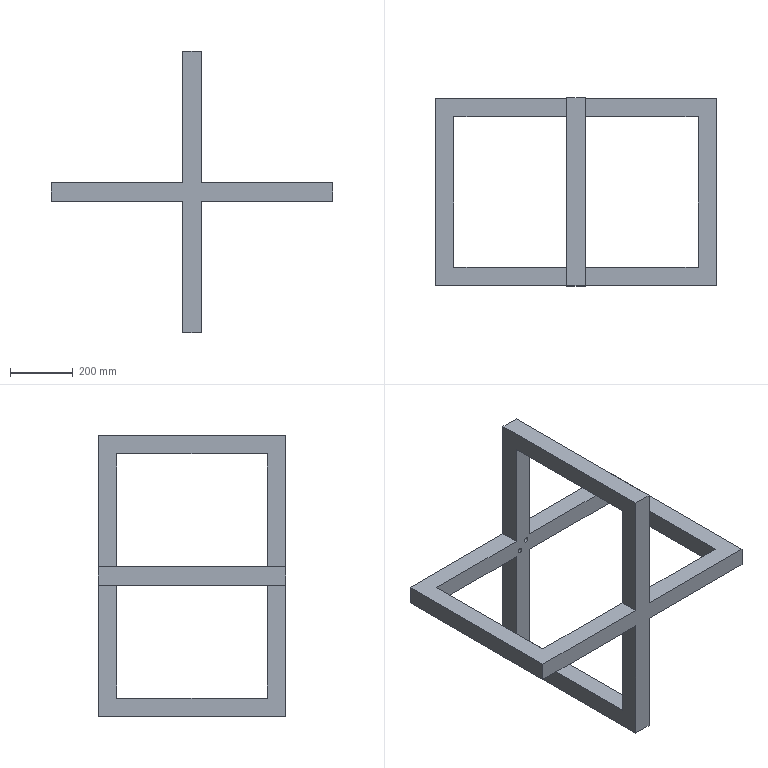Part | SolidWorks | features ICE 2, Extrusion 1, HoleWzd 1 | 1 solid | 27 faces | box 900 x 600 x 900 mm | volume 19278601 mm3 | plane 21 | cylinder 6 | commonest cylinder face diameters 15 x4 80 x2
STEP:
#1=CARTESIAN_POINT('',(-14.142,240.,-6.642));
#2=VERTEX_POINT('',#1);
#3=CARTESIAN_POINT('',(-14.142,240.,-21.642));
#4=VERTEX_POINT('',#3);
#5=CARTESIAN_POINT('',(-14.142,240.,-14.142));
#6=DIRECTION('',(0.,-1.,0.));
#7=DIRECTION('',(1.,0.,0.));
#8=AXIS2_PLACEMENT_3D('',#5,#6,#7);
#9=CIRCLE('',#8,7.5);
#10=EDGE_CURVE('',#2,#4,#9,.T.);
#11=ORIENTED_EDGE('',*,*,#10,.T.);
#12=CARTESIAN_POINT('',(-14.142,270.,-21.642));
#13=VERTEX_POINT('',#12);
#14=CARTESIAN_POINT('',(-14.142,270.,-21.642));
#15=DIRECTION('',(0.,1.,0.));
#16=VECTOR('',#15,1000.);
#17=LINE('',#14,#16);
#18=EDGE_CURVE('',#4,#13,#17,.T.);
#19=ORIENTED_EDGE('',*,*,#18,.T.);
#20=CARTESIAN_POINT('',(-14.142,270.,-6.642));
#21=VERTEX_POINT('',#20);
#22=CARTESIAN_POINT('',(-14.142,270.,-14.142));
#23=DIRECTION('',(0.,1.,0.));
#24=DIRECTION('',(0.,0.,1.));
#25=AXIS2_PLACEMENT_3D('',#22,#23,#24);
#26=CIRCLE('',#25,7.5);
#27=EDGE_CURVE('',#13,#21,#26,.T.);
#28=ORIENTED_EDGE('',*,*,#27,.T.);
#29=CARTESIAN_POINT('',(-14.142,270.,-6.642));
#30=DIRECTION('',(0.,1.,0.));
#31=VECTOR('',#30,1000.);
#32=LINE('',#29,#31);
#33=EDGE_CURVE('',#2,#21,#32,.T.);
#34=ORIENTED_EDGE('',*,*,#33,.F.);
#35=EDGE_LOOP('',(#11,#19,#28,#34));
#36=FACE_OUTER_BOUND('',#35,.T.);
#37=CARTESIAN_POINT('',(-14.142,270.,-14.142));
#38=DIRECTION('',(0.,1.,0.));
#39=DIRECTION('',(0.,0.,1.));
#40=AXIS2_PLACEMENT_3D('',#37,#38,#39);
#41=CYLINDRICAL_SURFACE('',#40,7.5);
#42=ADVANCED_FACE('',(#36),#41,.F.);
#43=CARTESIAN_POINT('',(14.142,240.,21.642));
#44=VERTEX_POINT('',#43);
#45=CARTESIAN_POINT('',(14.142,240.,6.642));
#46=VERTEX_POINT('',#45);
#47=CARTESIAN_POINT('',(14.142,240.,14.142));
#48=DIRECTION('',(0.,-1.,0.));
#49=DIRECTION('',(1.,0.,0.));
#50=AXIS2_PLACEMENT_3D('',#47,#48,#49);
#51=CIRCLE('',#50,7.5);
#52=EDGE_CURVE('',#44,#46,#51,.T.);
#53=ORIENTED_EDGE('',*,*,#52,.T.);
#54=CARTESIAN_POINT('',(14.142,270.,6.642));
#55=VERTEX_POINT('',#54);
#56=CARTESIAN_POINT('',(14.142,270.,6.642));
#57=DIRECTION('',(0.,1.,0.));
#58=VECTOR('',#57,1000.);
#59=LINE('',#56,#58);
#60=EDGE_CURVE('',#46,#55,#59,.T.);
#61=ORIENTED_EDGE('',*,*,#60,.T.);
#62=CARTESIAN_POINT('',(14.142,270.,21.642));
#63=VERTEX_POINT('',#62);
#64=CARTESIAN_POINT('',(14.142,270.,14.142));
#65=DIRECTION('',(0.,1.,0.));
#66=DIRECTION('',(0.,0.,1.));
#67=AXIS2_PLACEMENT_3D('',#64,#65,#66);
#68=CIRCLE('',#67,7.5);
#69=EDGE_CURVE('',#55,#63,#68,.T.);
#70=ORIENTED_EDGE('',*,*,#69,.T.);
#71=CARTESIAN_POINT('',(14.142,270.,21.642));
#72=DIRECTION('',(0.,1.,0.));
#73=VECTOR('',#72,1000.);
#74=LINE('',#71,#73);
#75=EDGE_CURVE('',#44,#63,#74,.T.);
#76=ORIENTED_EDGE('',*,*,#75,.F.);
#77=EDGE_LOOP('',(#53,#61,#70,#76));
#78=FACE_OUTER_BOUND('',#77,.T.);
#79=CARTESIAN_POINT('',(14.142,270.,14.142));
#80=DIRECTION('',(0.,1.,0.));
#81=DIRECTION('',(0.,0.,1.));
#82=AXIS2_PLACEMENT_3D('',#79,#80,#81);
#83=CYLINDRICAL_SURFACE('',#82,7.5);
#84=ADVANCED_FACE('',(#78),#83,.F.);
#85=CARTESIAN_POINT('',(0.,270.,-40.));
#86=VERTEX_POINT('',#85);
#87=CARTESIAN_POINT('',(0.,270.,40.));
#88=VERTEX_POINT('',#87);
#89=CARTESIAN_POINT('',(0.,270.,0.));
#90=DIRECTION('',(0.,1.,0.));
#91=DIRECTION('',(0.,0.,1.));
#92=AXIS2_PLACEMENT_3D('',#89,#90,#91);
#93=CIRCLE('',#92,40.);
#94=EDGE_CURVE('',#86,#88,#93,.T.);
#95=ORIENTED_EDGE('',*,*,#94,.F.);
#96=CARTESIAN_POINT('',(0.,300.,-40.));
#97=VERTEX_POINT('',#96);
#98=CARTESIAN_POINT('',(0.,270.,-40.));
#99=DIRECTION('',(0.,1.,0.));
#100=VECTOR('',#99,1000.);
#101=LINE('',#98,#100);
#102=EDGE_CURVE('',#86,#97,#101,.T.);
#103=ORIENTED_EDGE('',*,*,#102,.T.);
#104=CARTESIAN_POINT('',(0.,300.,40.));
#105=VERTEX_POINT('',#104);
#106=CARTESIAN_POINT('',(0.,300.,0.));
#107=DIRECTION('',(0.,1.,0.));
#108=DIRECTION('',(0.,0.,1.));
#109=AXIS2_PLACEMENT_3D('',#106,#107,#108);
#110=CIRCLE('',#109,40.);
#111=EDGE_CURVE('',#97,#105,#110,.T.);
#112=ORIENTED_EDGE('',*,*,#111,.T.);
#113=CARTESIAN_POINT('',(0.,270.,40.));
#114=DIRECTION('',(0.,1.,0.));
#115=VECTOR('',#114,1000.);
#116=LINE('',#113,#115);
#117=EDGE_CURVE('',#88,#105,#116,.T.);
#118=ORIENTED_EDGE('',*,*,#117,.F.);
#119=EDGE_LOOP('',(#95,#103,#112,#118));
#120=FACE_OUTER_BOUND('',#119,.T.);
#121=CARTESIAN_POINT('',(0.,270.,0.));
#122=DIRECTION('',(0.,1.,0.));
#123=DIRECTION('',(0.,0.,1.));
#124=AXIS2_PLACEMENT_3D('',#121,#122,#123);
#125=CYLINDRICAL_SURFACE('',#124,40.);
#126=ADVANCED_FACE('',(#120),#125,.F.);
#127=CARTESIAN_POINT('',(30.,-300.,30.));
#128=VERTEX_POINT('',#127);
#129=CARTESIAN_POINT('',(30.,-240.,30.));
#130=VERTEX_POINT('',#129);
#131=CARTESIAN_POINT('',(30.,0.,30.));
#132=DIRECTION('',(0.,1.,0.));
#133=VECTOR('',#132,1000.);
#134=LINE('',#131,#133);
#135=EDGE_CURVE('',#128,#130,#134,.T.);
#136=ORIENTED_EDGE('',*,*,#135,.F.);
#137=CARTESIAN_POINT('',(450.,-300.,30.));
#138=VERTEX_POINT('',#137);
#139=CARTESIAN_POINT('',(-450.,-300.,30.));
#140=DIRECTION('',(1.,0.,0.));
#141=VECTOR('',#140,1000.);
#142=LINE('',#139,#141);
#143=EDGE_CURVE('',#128,#138,#142,.T.);
#144=ORIENTED_EDGE('',*,*,#143,.T.);
#145=CARTESIAN_POINT('',(450.,300.,30.));
#146=VERTEX_POINT('',#145);
#147=CARTESIAN_POINT('',(450.,-300.,30.));
#148=DIRECTION('',(0.,1.,0.));
#149=VECTOR('',#148,1000.);
#150=LINE('',#147,#149);
#151=EDGE_CURVE('',#138,#146,#150,.T.);
#152=ORIENTED_EDGE('',*,*,#151,.T.);
#153=CARTESIAN_POINT('',(30.,300.,30.));
#154=VERTEX_POINT('',#153);
#155=CARTESIAN_POINT('',(-450.,300.,30.));
#156=DIRECTION('',(-1.,0.,0.));
#157=VECTOR('',#156,1000.);
#158=LINE('',#155,#157);
#159=EDGE_CURVE('',#146,#154,#158,.T.);
#160=ORIENTED_EDGE('',*,*,#159,.T.);
#161=CARTESIAN_POINT('',(30.,240.,30.));
#162=VERTEX_POINT('',#161);
#163=CARTESIAN_POINT('',(30.,0.,30.));
#164=DIRECTION('',(0.,1.,0.));
#165=VECTOR('',#164,1000.);
#166=LINE('',#163,#165);
#167=EDGE_CURVE('',#162,#154,#166,.T.);
#168=ORIENTED_EDGE('',*,*,#167,.F.);
#169=CARTESIAN_POINT('',(390.,240.,30.));
#170=VERTEX_POINT('',#169);
#171=CARTESIAN_POINT('',(-390.,240.,30.));
#172=DIRECTION('',(-1.,0.,0.));
#173=VECTOR('',#172,1000.);
#174=LINE('',#171,#173);
#175=EDGE_CURVE('',#170,#162,#174,.T.);
#176=ORIENTED_EDGE('',*,*,#175,.F.);
#177=CARTESIAN_POINT('',(390.,-240.,30.));
#178=VERTEX_POINT('',#177);
#179=CARTESIAN_POINT('',(390.,-240.,30.));
#180=DIRECTION('',(0.,1.,0.));
#181=VECTOR('',#180,1000.);
#182=LINE('',#179,#181);
#183=EDGE_CURVE('',#178,#170,#182,.T.);
#184=ORIENTED_EDGE('',*,*,#183,.F.);
#185=CARTESIAN_POINT('',(-390.,-240.,30.));
#186=DIRECTION('',(1.,0.,0.));
#187=VECTOR('',#186,1000.);
#188=LINE('',#185,#187);
#189=EDGE_CURVE('',#130,#178,#188,.T.);
#190=ORIENTED_EDGE('',*,*,#189,.F.);
#191=EDGE_LOOP('',(#136,#144,#152,#160,#168,#176,#184,#190));
#192=FACE_OUTER_BOUND('',#191,.T.);
#193=CARTESIAN_POINT('',(0.,0.,30.));
#194=DIRECTION('',(0.,0.,-1.));
#195=DIRECTION('',(-1.,0.,0.));
#196=AXIS2_PLACEMENT_3D('',#193,#194,#195);
#197=PLANE('',#196);
#198=ADVANCED_FACE('',(#192),#197,.F.);
#199=CARTESIAN_POINT('',(30.,-300.,-30.));
#200=VERTEX_POINT('',#199);
#201=CARTESIAN_POINT('',(450.,-300.,-30.));
#202=VERTEX_POINT('',#201);
#203=CARTESIAN_POINT('',(-450.,-300.,-30.));
#204=DIRECTION('',(1.,0.,0.));
#205=VECTOR('',#204,1000.);
#206=LINE('',#203,#205);
#207=EDGE_CURVE('',#200,#202,#206,.T.);
#208=ORIENTED_EDGE('',*,*,#207,.F.);
#209=CARTESIAN_POINT('',(30.,-240.,-30.));
#210=VERTEX_POINT('',#209);
#211=CARTESIAN_POINT('',(30.,0.,-30.));
#212=DIRECTION('',(0.,1.,0.));
#213=VECTOR('',#212,1000.);
#214=LINE('',#211,#213);
#215=EDGE_CURVE('',#200,#210,#214,.T.);
#216=ORIENTED_EDGE('',*,*,#215,.T.);
#217=CARTESIAN_POINT('',(390.,-240.,-30.));
#218=VERTEX_POINT('',#217);
#219=CARTESIAN_POINT('',(-390.,-240.,-30.));
#220=DIRECTION('',(1.,0.,0.));
#221=VECTOR('',#220,1000.);
#222=LINE('',#219,#221);
#223=EDGE_CURVE('',#210,#218,#222,.T.);
#224=ORIENTED_EDGE('',*,*,#223,.T.);
#225=CARTESIAN_POINT('',(390.,240.,-30.));
#226=VERTEX_POINT('',#225);
#227=CARTESIAN_POINT('',(390.,-240.,-30.));
#228=DIRECTION('',(0.,1.,0.));
#229=VECTOR('',#228,1000.);
#230=LINE('',#227,#229);
#231=EDGE_CURVE('',#218,#226,#230,.T.);
#232=ORIENTED_EDGE('',*,*,#231,.T.);
#233=CARTESIAN_POINT('',(30.,240.,-30.));
#234=VERTEX_POINT('',#233);
#235=CARTESIAN_POINT('',(-390.,240.,-30.));
#236=DIRECTION('',(-1.,0.,0.));
#237=VECTOR('',#236,1000.);
#238=LINE('',#235,#237);
#239=EDGE_CURVE('',#226,#234,#238,.T.);
#240=ORIENTED_EDGE('',*,*,#239,.T.);
#241=CARTESIAN_POINT('',(30.,300.,-30.));
#242=VERTEX_POINT('',#241);
#243=CARTESIAN_POINT('',(30.,0.,-30.));
#244=DIRECTION('',(0.,1.,0.));
#245=VECTOR('',#244,1000.);
#246=LINE('',#243,#245);
#247=EDGE_CURVE('',#234,#242,#246,.T.);
#248=ORIENTED_EDGE('',*,*,#247,.T.);
#249=CARTESIAN_POINT('',(450.,300.,-30.));
#250=VERTEX_POINT('',#249);
#251=CARTESIAN_POINT('',(-450.,300.,-30.));
#252=DIRECTION('',(-1.,0.,0.));
#253=VECTOR('',#252,1000.);
#254=LINE('',#251,#253);
#255=EDGE_CURVE('',#250,#242,#254,.T.);
#256=ORIENTED_EDGE('',*,*,#255,.F.);
#257=CARTESIAN_POINT('',(450.,-300.,-30.));
#258=DIRECTION('',(0.,1.,0.));
#259=VECTOR('',#258,1000.);
#260=LINE('',#257,#259);
#261=EDGE_CURVE('',#202,#250,#260,.T.);
#262=ORIENTED_EDGE('',*,*,#261,.F.);
#263=EDGE_LOOP('',(#208,#216,#224,#232,#240,#248,#256,#262));
#264=FACE_OUTER_BOUND('',#263,.T.);
#265=CARTESIAN_POINT('',(0.,0.,-30.));
#266=DIRECTION('',(0.,0.,-1.));
#267=DIRECTION('',(-1.,0.,0.));
#268=AXIS2_PLACEMENT_3D('',#265,#266,#267);
#269=PLANE('',#268);
#270=ADVANCED_FACE('',(#264),#269,.T.);
#271=CARTESIAN_POINT('',(-450.,-300.,30.));
#272=VERTEX_POINT('',#271);
#273=CARTESIAN_POINT('',(-30.,-300.,30.));
#274=VERTEX_POINT('',#273);
#275=CARTESIAN_POINT('',(-450.,-300.,30.));
#276=DIRECTION('',(1.,0.,0.));
#277=VECTOR('',#276,1000.);
#278=LINE('',#275,#277);
#279=EDGE_CURVE('',#272,#274,#278,.T.);
#280=ORIENTED_EDGE('',*,*,#279,.T.);
#281=CARTESIAN_POINT('',(-30.,-240.,30.));
#282=VERTEX_POINT('',#281);
#283=CARTESIAN_POINT('',(-30.,0.,30.));
#284=DIRECTION('',(0.,1.,0.));
#285=VECTOR('',#284,1000.);
#286=LINE('',#283,#285);
#287=EDGE_CURVE('',#274,#282,#286,.T.);
#288=ORIENTED_EDGE('',*,*,#287,.T.);
#289=CARTESIAN_POINT('',(-390.,-240.,30.));
#290=VERTEX_POINT('',#289);
#291=CARTESIAN_POINT('',(-390.,-240.,30.));
#292=DIRECTION('',(1.,0.,0.));
#293=VECTOR('',#292,1000.);
#294=LINE('',#291,#293);
#295=EDGE_CURVE('',#290,#282,#294,.T.);
#296=ORIENTED_EDGE('',*,*,#295,.F.);
#297=CARTESIAN_POINT('',(-390.,240.,30.));
#298=VERTEX_POINT('',#297);
#299=CARTESIAN_POINT('',(-390.,-240.,30.));
#300=DIRECTION('',(0.,-1.,0.));
#301=VECTOR('',#300,1000.);
#302=LINE('',#299,#301);
#303=EDGE_CURVE('',#298,#290,#302,.T.);
#304=ORIENTED_EDGE('',*,*,#303,.F.);
#305=CARTESIAN_POINT('',(-30.,240.,30.));
#306=VERTEX_POINT('',#305);
#307=CARTESIAN_POINT('',(-390.,240.,30.));
#308=DIRECTION('',(-1.,0.,0.));
#309=VECTOR('',#308,1000.);
#310=LINE('',#307,#309);
#311=EDGE_CURVE('',#306,#298,#310,.T.);
#312=ORIENTED_EDGE('',*,*,#311,.F.);
#313=CARTESIAN_POINT('',(-30.,300.,30.));
#314=VERTEX_POINT('',#313);
#315=CARTESIAN_POINT('',(-30.,0.,30.));
#316=DIRECTION('',(0.,1.,0.));
#317=VECTOR('',#316,1000.);
#318=LINE('',#315,#317);
#319=EDGE_CURVE('',#306,#314,#318,.T.);
#320=ORIENTED_EDGE('',*,*,#319,.T.);
#321=CARTESIAN_POINT('',(-450.,300.,30.));
#322=VERTEX_POINT('',#321);
#323=CARTESIAN_POINT('',(-450.,300.,30.));
#324=DIRECTION('',(-1.,0.,0.));
#325=VECTOR('',#324,1000.);
#326=LINE('',#323,#325);
#327=EDGE_CURVE('',#314,#322,#326,.T.);
#328=ORIENTED_EDGE('',*,*,#327,.T.);
#329=CARTESIAN_POINT('',(-450.,-300.,30.));
#330=DIRECTION('',(0.,-1.,0.));
#331=VECTOR('',#330,1000.);
#332=LINE('',#329,#331);
#333=EDGE_CURVE('',#322,#272,#332,.T.);
#334=ORIENTED_EDGE('',*,*,#333,.T.);
#335=EDGE_LOOP('',(#280,#288,#296,#304,#312,#320,#328,#334));
#336=FACE_OUTER_BOUND('',#335,.T.);
#337=CARTESIAN_POINT('',(0.,0.,30.));
#338=DIRECTION('',(0.,0.,-1.));
#339=DIRECTION('',(-1.,0.,0.));
#340=AXIS2_PLACEMENT_3D('',#337,#338,#339);
#341=PLANE('',#340);
#342=ADVANCED_FACE('',(#336),#341,.F.);
#343=CARTESIAN_POINT('',(-30.,-300.,-30.));
#344=VERTEX_POINT('',#343);
#345=CARTESIAN_POINT('',(-30.,-240.,-30.));
#346=VERTEX_POINT('',#345);
#347=CARTESIAN_POINT('',(-30.,0.,-30.));
#348=DIRECTION('',(0.,1.,0.));
#349=VECTOR('',#348,1000.);
#350=LINE('',#347,#349);
#351=EDGE_CURVE('',#344,#346,#350,.T.);
#352=ORIENTED_EDGE('',*,*,#351,.F.);
#353=CARTESIAN_POINT('',(-450.,-300.,-30.));
#354=VERTEX_POINT('',#353);
#355=CARTESIAN_POINT('',(-450.,-300.,-30.));
#356=DIRECTION('',(1.,0.,0.));
#357=VECTOR('',#356,1000.);
#358=LINE('',#355,#357);
#359=EDGE_CURVE('',#354,#344,#358,.T.);
#360=ORIENTED_EDGE('',*,*,#359,.F.);
#361=CARTESIAN_POINT('',(-450.,300.,-30.));
#362=VERTEX_POINT('',#361);
#363=CARTESIAN_POINT('',(-450.,-300.,-30.));
#364=DIRECTION('',(0.,-1.,0.));
#365=VECTOR('',#364,1000.);
#366=LINE('',#363,#365);
#367=EDGE_CURVE('',#362,#354,#366,.T.);
#368=ORIENTED_EDGE('',*,*,#367,.F.);
#369=CARTESIAN_POINT('',(-30.,300.,-30.));
#370=VERTEX_POINT('',#369);
#371=CARTESIAN_POINT('',(-450.,300.,-30.));
#372=DIRECTION('',(-1.,0.,0.));
#373=VECTOR('',#372,1000.);
#374=LINE('',#371,#373);
#375=EDGE_CURVE('',#370,#362,#374,.T.);
#376=ORIENTED_EDGE('',*,*,#375,.F.);
#377=CARTESIAN_POINT('',(-30.,240.,-30.));
#378=VERTEX_POINT('',#377);
#379=CARTESIAN_POINT('',(-30.,0.,-30.));
#380=DIRECTION('',(0.,1.,0.));
#381=VECTOR('',#380,1000.);
#382=LINE('',#379,#381);
#383=EDGE_CURVE('',#378,#370,#382,.T.);
#384=ORIENTED_EDGE('',*,*,#383,.F.);
#385=CARTESIAN_POINT('',(-390.,240.,-30.));
#386=VERTEX_POINT('',#385);
#387=CARTESIAN_POINT('',(-390.,240.,-30.));
#388=DIRECTION('',(-1.,0.,0.));
#389=VECTOR('',#388,1000.);
#390=LINE('',#387,#389);
#391=EDGE_CURVE('',#378,#386,#390,.T.);
#392=ORIENTED_EDGE('',*,*,#391,.T.);
#393=CARTESIAN_POINT('',(-390.,-240.,-30.));
#394=VERTEX_POINT('',#393);
#395=CARTESIAN_POINT('',(-390.,-240.,-30.));
#396=DIRECTION('',(0.,-1.,0.));
#397=VECTOR('',#396,1000.);
#398=LINE('',#395,#397);
#399=EDGE_CURVE('',#386,#394,#398,.T.);
#400=ORIENTED_EDGE('',*,*,#399,.T.);
#401=CARTESIAN_POINT('',(-390.,-240.,-30.));
#402=DIRECTION('',(1.,0.,0.));
#403=VECTOR('',#402,1000.);
#404=LINE('',#401,#403);
#405=EDGE_CURVE('',#394,#346,#404,.T.);
#406=ORIENTED_EDGE('',*,*,#405,.T.);
#407=EDGE_LOOP('',(#352,#360,#368,#376,#384,#392,#400,#406));
#408=FACE_OUTER_BOUND('',#407,.T.);
#409=CARTESIAN_POINT('',(0.,0.,-30.));
#410=DIRECTION('',(0.,0.,-1.));
#411=DIRECTION('',(-1.,0.,0.));
#412=AXIS2_PLACEMENT_3D('',#409,#410,#411);
#413=PLANE('',#412);
#414=ADVANCED_FACE('',(#408),#413,.T.);
#415=ORIENTED_EDGE('',*,*,#367,.T.);
#416=CARTESIAN_POINT('',(-450.,-300.,30.));
#417=DIRECTION('',(0.,0.,-1.));
#418=VECTOR('',#417,1000.);
#419=LINE('',#416,#418);
#420=EDGE_CURVE('',#272,#354,#419,.T.);
#421=ORIENTED_EDGE('',*,*,#420,.F.);
#422=ORIENTED_EDGE('',*,*,#333,.F.);
#423=CARTESIAN_POINT('',(-450.,300.,30.));
#424=DIRECTION('',(0.,0.,-1.));
#425=VECTOR('',#424,1000.);
#426=LINE('',#423,#425);
#427=EDGE_CURVE('',#322,#362,#426,.T.);
#428=ORIENTED_EDGE('',*,*,#427,.T.);
#429=EDGE_LOOP('',(#415,#421,#422,#428));
#430=FACE_OUTER_BOUND('',#429,.T.);
#431=CARTESIAN_POINT('',(-450.,-300.,30.));
#432=DIRECTION('',(1.,0.,0.));
#433=DIRECTION('',(0.,0.,-1.));
#434=AXIS2_PLACEMENT_3D('',#431,#432,#433);
#435=PLANE('',#434);
#436=ADVANCED_FACE('',(#430),#435,.F.);
#437=ORIENTED_EDGE('',*,*,#359,.T.);
#438=CARTESIAN_POINT('',(-30.,-300.,-450.));
#439=VERTEX_POINT('',#438);
#440=CARTESIAN_POINT('',(-30.,-300.,450.));
#441=DIRECTION('',(0.,0.,-1.));
#442=VECTOR('',#441,1000.);
#443=LINE('',#440,#442);
#444=EDGE_CURVE('',#344,#439,#443,.T.);
#445=ORIENTED_EDGE('',*,*,#444,.T.);
#446=CARTESIAN_POINT('',(30.,-300.,-450.));
#447=VERTEX_POINT('',#446);
#448=CARTESIAN_POINT('',(30.,-300.,-450.));
#449=DIRECTION('',(-1.,0.,0.));
#450=VECTOR('',#449,1000.);
#451=LINE('',#448,#450);
#452=EDGE_CURVE('',#447,#439,#451,.T.);
#453=ORIENTED_EDGE('',*,*,#452,.F.);
#454=CARTESIAN_POINT('',(30.,-300.,450.));
#455=DIRECTION('',(0.,0.,-1.));
#456=VECTOR('',#455,1000.);
#457=LINE('',#454,#456);
#458=EDGE_CURVE('',#200,#447,#457,.T.);
#459=ORIENTED_EDGE('',*,*,#458,.F.);
#460=ORIENTED_EDGE('',*,*,#207,.T.);
#461=CARTESIAN_POINT('',(450.,-300.,30.));
#462=DIRECTION('',(0.,0.,-1.));
#463=VECTOR('',#462,1000.);
#464=LINE('',#461,#463);
#465=EDGE_CURVE('',#138,#202,#464,.T.);
#466=ORIENTED_EDGE('',*,*,#465,.F.);
#467=ORIENTED_EDGE('',*,*,#143,.F.);
#468=CARTESIAN_POINT('',(30.,-300.,450.));
#469=VERTEX_POINT('',#468);
#470=CARTESIAN_POINT('',(30.,-300.,450.));
#471=DIRECTION('',(0.,0.,-1.));
#472=VECTOR('',#471,1000.);
#473=LINE('',#470,#472);
#474=EDGE_CURVE('',#469,#128,#473,.T.);
#475=ORIENTED_EDGE('',*,*,#474,.F.);
#476=CARTESIAN_POINT('',(-30.,-300.,450.));
#477=VERTEX_POINT('',#476);
#478=CARTESIAN_POINT('',(30.,-300.,450.));
#479=DIRECTION('',(-1.,0.,0.));
#480=VECTOR('',#479,1000.);
#481=LINE('',#478,#480);
#482=EDGE_CURVE('',#469,#477,#481,.T.);
#483=ORIENTED_EDGE('',*,*,#482,.T.);
#484=CARTESIAN_POINT('',(-30.,-300.,450.));
#485=DIRECTION('',(0.,0.,-1.));
#486=VECTOR('',#485,1000.);
#487=LINE('',#484,#486);
#488=EDGE_CURVE('',#477,#274,#487,.T.);
#489=ORIENTED_EDGE('',*,*,#488,.T.);
#490=ORIENTED_EDGE('',*,*,#279,.F.);
#491=ORIENTED_EDGE('',*,*,#420,.T.);
#492=EDGE_LOOP('',(#437,#445,#453,#459,#460,#466,#467,#475,#483,#489,#490,#491));
#493=FACE_OUTER_BOUND('',#492,.T.);
#494=CARTESIAN_POINT('',(-450.,-300.,30.));
#495=DIRECTION('',(0.,1.,0.));
#496=DIRECTION('',(0.,0.,1.));
#497=AXIS2_PLACEMENT_3D('',#494,#495,#496);
#498=PLANE('',#497);
#499=ADVANCED_FACE('',(#493),#498,.F.);
#500=ORIENTED_EDGE('',*,*,#261,.T.);
#501=CARTESIAN_POINT('',(450.,300.,30.));
#502=DIRECTION('',(0.,0.,-1.));
#503=VECTOR('',#502,1000.);
#504=LINE('',#501,#503);
#505=EDGE_CURVE('',#146,#250,#504,.T.);
#506=ORIENTED_EDGE('',*,*,#505,.F.);
#507=ORIENTED_EDGE('',*,*,#151,.F.);
#508=ORIENTED_EDGE('',*,*,#465,.T.);
#509=EDGE_LOOP('',(#500,#506,#507,#508));
#510=FACE_OUTER_BOUND('',#509,.T.);
#511=CARTESIAN_POINT('',(450.,-300.,30.));
#512=DIRECTION('',(-1.,0.,0.));
#513=DIRECTION('',(0.,0.,1.));
#514=AXIS2_PLACEMENT_3D('',#511,#512,#513);
#515=PLANE('',#514);
#516=ADVANCED_FACE('',(#510),#515,.F.);
#517=CARTESIAN_POINT('',(0.,300.,0.));
#518=DIRECTION('',(0.,1.,0.));
#519=DIRECTION('',(0.,0.,1.));
#520=AXIS2_PLACEMENT_3D('',#517,#518,#519);
#521=CIRCLE('',#520,40.);
#522=EDGE_CURVE('',#105,#97,#521,.T.);
#523=ORIENTED_EDGE('',*,*,#522,.F.);
#524=ORIENTED_EDGE('',*,*,#111,.F.);
#525=EDGE_LOOP('',(#523,#524));
#526=FACE_BOUND('',#525,.T.);
#527=ORIENTED_EDGE('',*,*,#327,.F.);
#528=CARTESIAN_POINT('',(-30.,300.,450.));
#529=VERTEX_POINT('',#528);
#530=CARTESIAN_POINT('',(-30.,300.,450.));
#531=DIRECTION('',(0.,0.,1.));
#532=VECTOR('',#531,1000.);
#533=LINE('',#530,#532);
#534=EDGE_CURVE('',#314,#529,#533,.T.);
#535=ORIENTED_EDGE('',*,*,#534,.T.);
#536=CARTESIAN_POINT('',(30.,300.,450.));
#537=VERTEX_POINT('',#536);
#538=CARTESIAN_POINT('',(30.,300.,450.));
#539=DIRECTION('',(-1.,0.,0.));
#540=VECTOR('',#539,1000.);
#541=LINE('',#538,#540);
#542=EDGE_CURVE('',#537,#529,#541,.T.);
#543=ORIENTED_EDGE('',*,*,#542,.F.);
#544=CARTESIAN_POINT('',(30.,300.,450.));
#545=DIRECTION('',(0.,0.,1.));
#546=VECTOR('',#545,1000.);
#547=LINE('',#544,#546);
#548=EDGE_CURVE('',#154,#537,#547,.T.);
#549=ORIENTED_EDGE('',*,*,#548,.F.);
#550=ORIENTED_EDGE('',*,*,#159,.F.);
#551=ORIENTED_EDGE('',*,*,#505,.T.);
#552=ORIENTED_EDGE('',*,*,#255,.T.);
#553=CARTESIAN_POINT('',(30.,300.,-450.));
#554=VERTEX_POINT('',#553);
#555=CARTESIAN_POINT('',(30.,300.,450.));
#556=DIRECTION('',(0.,0.,1.));
#557=VECTOR('',#556,1000.);
#558=LINE('',#555,#557);
#559=EDGE_CURVE('',#554,#242,#558,.T.);
#560=ORIENTED_EDGE('',*,*,#559,.F.);
#561=CARTESIAN_POINT('',(-30.,300.,-450.));
#562=VERTEX_POINT('',#561);
#563=CARTESIAN_POINT('',(30.,300.,-450.));
#564=DIRECTION('',(-1.,0.,0.));
#565=VECTOR('',#564,1000.);
#566=LINE('',#563,#565);
#567=EDGE_CURVE('',#554,#562,#566,.T.);
#568=ORIENTED_EDGE('',*,*,#567,.T.);
#569=CARTESIAN_POINT('',(-30.,300.,450.));
#570=DIRECTION('',(0.,0.,1.));
#571=VECTOR('',#570,1000.);
#572=LINE('',#569,#571);
#573=EDGE_CURVE('',#562,#370,#572,.T.);
#574=ORIENTED_EDGE('',*,*,#573,.T.);
#575=ORIENTED_EDGE('',*,*,#375,.T.);
#576=ORIENTED_EDGE('',*,*,#427,.F.);
#577=EDGE_LOOP('',(#527,#535,#543,#549,#550,#551,#552,#560,#568,#574,#575,#576));
#578=FACE_OUTER_BOUND('',#577,.T.);
#579=CARTESIAN_POINT('',(-450.,300.,30.));
#580=DIRECTION('',(0.,-1.,0.));
#581=DIRECTION('',(0.,0.,-1.));
#582=AXIS2_PLACEMENT_3D('',#579,#580,#581);
#583=PLANE('',#582);
#584=ADVANCED_FACE('',(#526,#578),#583,.F.);
#585=ORIENTED_EDGE('',*,*,#231,.F.);
#586=CARTESIAN_POINT('',(390.,-240.,30.));
#587=DIRECTION('',(0.,0.,-1.));
#588=VECTOR('',#587,1000.);
#589=LINE('',#586,#588);
#590=EDGE_CURVE('',#178,#218,#589,.T.);
#591=ORIENTED_EDGE('',*,*,#590,.F.);
#592=ORIENTED_EDGE('',*,*,#183,.T.);
#593=CARTESIAN_POINT('',(390.,240.,30.));
#594=DIRECTION('',(0.,0.,-1.));
#595=VECTOR('',#594,1000.);
#596=LINE('',#593,#595);
#597=EDGE_CURVE('',#170,#226,#596,.T.);
#598=ORIENTED_EDGE('',*,*,#597,.T.);
#599=EDGE_LOOP('',(#585,#591,#592,#598));
#600=FACE_OUTER_BOUND('',#599,.T.);
#601=CARTESIAN_POINT('',(390.,-240.,30.));
#602=DIRECTION('',(-1.,0.,0.));
#603=DIRECTION('',(0.,0.,1.));
#604=AXIS2_PLACEMENT_3D('',#601,#602,#603);
#605=PLANE('',#604);
#606=ADVANCED_FACE('',(#600),#605,.T.);
#607=ORIENTED_EDGE('',*,*,#10,.F.);
#608=CARTESIAN_POINT('',(-14.142,240.,-14.142));
#609=DIRECTION('',(0.,-1.,0.));
#610=DIRECTION('',(1.,0.,0.));
#611=AXIS2_PLACEMENT_3D('',#608,#609,#610);
#612=CIRCLE('',#611,7.5);
#613=EDGE_CURVE('',#4,#2,#612,.T.);
#614=ORIENTED_EDGE('',*,*,#613,.F.);
#615=EDGE_LOOP('',(#607,#614));
#616=FACE_BOUND('',#615,.T.);
#617=ORIENTED_EDGE('',*,*,#52,.F.);
#618=CARTESIAN_POINT('',(14.142,240.,14.142));
#619=DIRECTION('',(0.,-1.,0.));
#620=DIRECTION('',(1.,0.,0.));
#621=AXIS2_PLACEMENT_3D('',#618,#619,#620);
#622=CIRCLE('',#621,7.5);
#623=EDGE_CURVE('',#46,#44,#622,.T.);
#624=ORIENTED_EDGE('',*,*,#623,.F.);
#625=EDGE_LOOP('',(#617,#624));
#626=FACE_BOUND('',#625,.T.);
#627=ORIENTED_EDGE('',*,*,#391,.F.);
#628=CARTESIAN_POINT('',(-30.,240.,-390.));
#629=VERTEX_POINT('',#628);
#630=CARTESIAN_POINT('',(-30.,240.,390.));
#631=DIRECTION('',(0.,0.,1.));
#632=VECTOR('',#631,1000.);
#633=LINE('',#630,#632);
#634=EDGE_CURVE('',#629,#378,#633,.T.);
#635=ORIENTED_EDGE('',*,*,#634,.F.);
#636=CARTESIAN_POINT('',(30.,240.,-390.));
#637=VERTEX_POINT('',#636);
#638=CARTESIAN_POINT('',(30.,240.,-390.));
#639=DIRECTION('',(-1.,0.,0.));
#640=VECTOR('',#639,1000.);
#641=LINE('',#638,#640);
#642=EDGE_CURVE('',#637,#629,#641,.T.);
#643=ORIENTED_EDGE('',*,*,#642,.F.);
#644=CARTESIAN_POINT('',(30.,240.,390.));
#645=DIRECTION('',(0.,0.,1.));
#646=VECTOR('',#645,1000.);
#647=LINE('',#644,#646);
#648=EDGE_CURVE('',#637,#234,#647,.T.);
#649=ORIENTED_EDGE('',*,*,#648,.T.);
#650=ORIENTED_EDGE('',*,*,#239,.F.);
#651=ORIENTED_EDGE('',*,*,#597,.F.);
#652=ORIENTED_EDGE('',*,*,#175,.T.);
#653=CARTESIAN_POINT('',(30.,240.,390.));
#654=VERTEX_POINT('',#653);
#655=CARTESIAN_POINT('',(30.,240.,390.));
#656=DIRECTION('',(0.,0.,1.));
#657=VECTOR('',#656,1000.);
#658=LINE('',#655,#657);
#659=EDGE_CURVE('',#162,#654,#658,.T.);
#660=ORIENTED_EDGE('',*,*,#659,.T.);
#661=CARTESIAN_POINT('',(-30.,240.,390.));
#662=VERTEX_POINT('',#661);
#663=CARTESIAN_POINT('',(30.,240.,390.));
#664=DIRECTION('',(-1.,0.,0.));
#665=VECTOR('',#664,1000.);
#666=LINE('',#663,#665);
#667=EDGE_CURVE('',#654,#662,#666,.T.);
#668=ORIENTED_EDGE('',*,*,#667,.T.);
#669=CARTESIAN_POINT('',(-30.,240.,390.));
#670=DIRECTION('',(0.,0.,1.));
#671=VECTOR('',#670,1000.);
#672=LINE('',#669,#671);
#673=EDGE_CURVE('',#306,#662,#672,.T.);
#674=ORIENTED_EDGE('',*,*,#673,.F.);
#675=ORIENTED_EDGE('',*,*,#311,.T.);
#676=CARTESIAN_POINT('',(-390.,240.,30.));
#677=DIRECTION('',(0.,0.,-1.));
#678=VECTOR('',#677,1000.);
#679=LINE('',#676,#678);
#680=EDGE_CURVE('',#298,#386,#679,.T.);
#681=ORIENTED_EDGE('',*,*,#680,.T.);
#682=EDGE_LOOP('',(#627,#635,#643,#649,#650,#651,#652,#660,#668,#674,#675,#681));
#683=FACE_OUTER_BOUND('',#682,.T.);
#684=CARTESIAN_POINT('',(-390.,240.,30.));
#685=DIRECTION('',(0.,-1.,0.));
#686=DIRECTION('',(1.,0.,0.));
#687=AXIS2_PLACEMENT_3D('',#684,#685,#686);
#688=PLANE('',#687);
#689=ADVANCED_FACE('',(#616,#626,#683),#688,.T.);
#690=ORIENTED_EDGE('',*,*,#399,.F.);
#691=ORIENTED_EDGE('',*,*,#680,.F.);
#692=ORIENTED_EDGE('',*,*,#303,.T.);
#693=CARTESIAN_POINT('',(-390.,-240.,30.));
#694=DIRECTION('',(0.,0.,-1.));
#695=VECTOR('',#694,1000.);
#696=LINE('',#693,#695);
#697=EDGE_CURVE('',#290,#394,#696,.T.);
#698=ORIENTED_EDGE('',*,*,#697,.T.);
#699=EDGE_LOOP('',(#690,#691,#692,#698));
#700=FACE_OUTER_BOUND('',#699,.T.);
#701=CARTESIAN_POINT('',(-390.,-240.,30.));
#702=DIRECTION('',(1.,0.,0.));
#703=DIRECTION('',(0.,1.,0.));
#704=AXIS2_PLACEMENT_3D('',#701,#702,#703);
#705=PLANE('',#704);
#706=ADVANCED_FACE('',(#700),#705,.T.);
#707=ORIENTED_EDGE('',*,*,#295,.T.);
#708=CARTESIAN_POINT('',(-30.,-240.,390.));
#709=VERTEX_POINT('',#708);
#710=CARTESIAN_POINT('',(-30.,-240.,390.));
#711=DIRECTION('',(0.,0.,-1.));
#712=VECTOR('',#711,1000.);
#713=LINE('',#710,#712);
#714=EDGE_CURVE('',#709,#282,#713,.T.);
#715=ORIENTED_EDGE('',*,*,#714,.F.);
#716=CARTESIAN_POINT('',(30.,-240.,390.));
#717=VERTEX_POINT('',#716);
#718=CARTESIAN_POINT('',(30.,-240.,390.));
#719=DIRECTION('',(-1.,0.,0.));
#720=VECTOR('',#719,1000.);
#721=LINE('',#718,#720);
#722=EDGE_CURVE('',#717,#709,#721,.T.);
#723=ORIENTED_EDGE('',*,*,#722,.F.);
#724=CARTESIAN_POINT('',(30.,-240.,390.));
#725=DIRECTION('',(0.,0.,-1.));
#726=VECTOR('',#725,1000.);
#727=LINE('',#724,#726);
#728=EDGE_CURVE('',#717,#130,#727,.T.);
#729=ORIENTED_EDGE('',*,*,#728,.T.);
#730=ORIENTED_EDGE('',*,*,#189,.T.);
#731=ORIENTED_EDGE('',*,*,#590,.T.);
#732=ORIENTED_EDGE('',*,*,#223,.F.);
#733=CARTESIAN_POINT('',(30.,-240.,-390.));
#734=VERTEX_POINT('',#733);
#735=CARTESIAN_POINT('',(30.,-240.,390.));
#736=DIRECTION('',(0.,0.,-1.));
#737=VECTOR('',#736,1000.);
#738=LINE('',#735,#737);
#739=EDGE_CURVE('',#210,#734,#738,.T.);
#740=ORIENTED_EDGE('',*,*,#739,.T.);
#741=CARTESIAN_POINT('',(-30.,-240.,-390.));
#742=VERTEX_POINT('',#741);
#743=CARTESIAN_POINT('',(30.,-240.,-390.));
#744=DIRECTION('',(-1.,0.,0.));
#745=VECTOR('',#744,1000.);
#746=LINE('',#743,#745);
#747=EDGE_CURVE('',#734,#742,#746,.T.);
#748=ORIENTED_EDGE('',*,*,#747,.T.);
#749=CARTESIAN_POINT('',(-30.,-240.,390.));
#750=DIRECTION('',(0.,0.,-1.));
#751=VECTOR('',#750,1000.);
#752=LINE('',#749,#751);
#753=EDGE_CURVE('',#346,#742,#752,.T.);
#754=ORIENTED_EDGE('',*,*,#753,.F.);
#755=ORIENTED_EDGE('',*,*,#405,.F.);
#756=ORIENTED_EDGE('',*,*,#697,.F.);
#757=EDGE_LOOP('',(#707,#715,#723,#729,#730,#731,#732,#740,#748,#754,#755,#756));
#758=FACE_OUTER_BOUND('',#757,.T.);
#759=CARTESIAN_POINT('',(-390.,-240.,30.));
#760=DIRECTION('',(0.,1.,0.));
#761=DIRECTION('',(-1.,0.,0.));
#762=AXIS2_PLACEMENT_3D('',#759,#760,#761);
#763=PLANE('',#762);
#764=ADVANCED_FACE('',(#758),#763,.T.);
#765=CARTESIAN_POINT('',(-30.,-300.,-450.));
#766=DIRECTION('',(0.,1.,0.));
#767=VECTOR('',#766,1000.);
#768=LINE('',#765,#767);
#769=EDGE_CURVE('',#439,#562,#768,.T.);
#770=ORIENTED_EDGE('',*,*,#769,.T.);
#771=ORIENTED_EDGE('',*,*,#567,.F.);
#772=CARTESIAN_POINT('',(30.,-300.,-450.));
#773=DIRECTION('',(0.,1.,0.));
#774=VECTOR('',#773,1000.);
#775=LINE('',#772,#774);
#776=EDGE_CURVE('',#447,#554,#775,.T.);
#777=ORIENTED_EDGE('',*,*,#776,.F.);
#778=ORIENTED_EDGE('',*,*,#452,.T.);
#779=EDGE_LOOP('',(#770,#771,#777,#778));
#780=FACE_OUTER_BOUND('',#779,.T.);
#781=CARTESIAN_POINT('',(30.,-300.,-450.));
#782=DIRECTION('',(0.,0.,1.));
#783=DIRECTION('',(1.,0.,0.));
#784=AXIS2_PLACEMENT_3D('',#781,#782,#783);
#785=PLANE('',#784);
#786=ADVANCED_FACE('',(#780),#785,.F.);
#787=CARTESIAN_POINT('',(-30.,-240.,-390.));
#788=DIRECTION('',(0.,1.,0.));
#789=VECTOR('',#788,1000.);
#790=LINE('',#787,#789);
#791=EDGE_CURVE('',#742,#629,#790,.T.);
#792=ORIENTED_EDGE('',*,*,#791,.F.);
#793=ORIENTED_EDGE('',*,*,#747,.F.);
#794=CARTESIAN_POINT('',(30.,-240.,-390.));
#795=DIRECTION('',(0.,1.,0.));
#796=VECTOR('',#795,1000.);
#797=LINE('',#794,#796);
#798=EDGE_CURVE('',#734,#637,#797,.T.);
#799=ORIENTED_EDGE('',*,*,#798,.T.);
#800=ORIENTED_EDGE('',*,*,#642,.T.);
#801=EDGE_LOOP('',(#792,#793,#799,#800));
#802=FACE_OUTER_BOUND('',#801,.T.);
#803=CARTESIAN_POINT('',(30.,-240.,-390.));
#804=DIRECTION('',(0.,0.,1.));
#805=DIRECTION('',(1.,0.,0.));
#806=AXIS2_PLACEMENT_3D('',#803,#804,#805);
#807=PLANE('',#806);
#808=ADVANCED_FACE('',(#802),#807,.T.);
#809=ORIENTED_EDGE('',*,*,#444,.F.);
#810=ORIENTED_EDGE('',*,*,#351,.T.);
#811=ORIENTED_EDGE('',*,*,#753,.T.);
#812=ORIENTED_EDGE('',*,*,#791,.T.);
#813=ORIENTED_EDGE('',*,*,#634,.T.);
#814=ORIENTED_EDGE('',*,*,#383,.T.);
#815=ORIENTED_EDGE('',*,*,#573,.F.);
#816=ORIENTED_EDGE('',*,*,#769,.F.);
#817=EDGE_LOOP('',(#809,#810,#811,#812,#813,#814,#815,#816));
#818=FACE_OUTER_BOUND('',#817,.T.);
#819=CARTESIAN_POINT('',(-30.,0.,0.));
#820=DIRECTION('',(-1.,0.,0.));
#821=DIRECTION('',(0.,0.,1.));
#822=AXIS2_PLACEMENT_3D('',#819,#820,#821);
#823=PLANE('',#822);
#824=ADVANCED_FACE('',(#818),#823,.T.);
#825=ORIENTED_EDGE('',*,*,#215,.F.);
#826=ORIENTED_EDGE('',*,*,#458,.T.);
#827=ORIENTED_EDGE('',*,*,#776,.T.);
#828=ORIENTED_EDGE('',*,*,#559,.T.);
#829=ORIENTED_EDGE('',*,*,#247,.F.);
#830=ORIENTED_EDGE('',*,*,#648,.F.);
#831=ORIENTED_EDGE('',*,*,#798,.F.);
#832=ORIENTED_EDGE('',*,*,#739,.F.);
#833=EDGE_LOOP('',(#825,#826,#827,#828,#829,#830,#831,#832));
#834=FACE_OUTER_BOUND('',#833,.T.);
#835=CARTESIAN_POINT('',(30.,0.,0.));
#836=DIRECTION('',(-1.,0.,0.));
#837=DIRECTION('',(0.,0.,1.));
#838=AXIS2_PLACEMENT_3D('',#835,#836,#837);
#839=PLANE('',#838);
#840=ADVANCED_FACE('',(#834),#839,.F.);
#841=ORIENTED_EDGE('',*,*,#474,.T.);
#842=ORIENTED_EDGE('',*,*,#135,.T.);
#843=ORIENTED_EDGE('',*,*,#728,.F.);
#844=CARTESIAN_POINT('',(30.,-240.,390.));
#845=DIRECTION('',(0.,-1.,0.));
#846=VECTOR('',#845,1000.);
#847=LINE('',#844,#846);
#848=EDGE_CURVE('',#654,#717,#847,.T.);
#849=ORIENTED_EDGE('',*,*,#848,.F.);
#850=ORIENTED_EDGE('',*,*,#659,.F.);
#851=ORIENTED_EDGE('',*,*,#167,.T.);
#852=ORIENTED_EDGE('',*,*,#548,.T.);
#853=CARTESIAN_POINT('',(30.,-300.,450.));
#854=DIRECTION('',(0.,-1.,0.));
#855=VECTOR('',#854,1000.);
#856=LINE('',#853,#855);
#857=EDGE_CURVE('',#537,#469,#856,.T.);
#858=ORIENTED_EDGE('',*,*,#857,.T.);
#859=EDGE_LOOP('',(#841,#842,#843,#849,#850,#851,#852,#858));
#860=FACE_OUTER_BOUND('',#859,.T.);
#861=CARTESIAN_POINT('',(30.,0.,0.));
#862=DIRECTION('',(-1.,0.,0.));
#863=DIRECTION('',(0.,0.,1.));
#864=AXIS2_PLACEMENT_3D('',#861,#862,#863);
#865=PLANE('',#864);
#866=ADVANCED_FACE('',(#860),#865,.F.);
#867=ORIENTED_EDGE('',*,*,#287,.F.);
#868=ORIENTED_EDGE('',*,*,#488,.F.);
#869=CARTESIAN_POINT('',(-30.,-300.,450.));
#870=DIRECTION('',(0.,-1.,0.));
#871=VECTOR('',#870,1000.);
#872=LINE('',#869,#871);
#873=EDGE_CURVE('',#529,#477,#872,.T.);
#874=ORIENTED_EDGE('',*,*,#873,.F.);
#875=ORIENTED_EDGE('',*,*,#534,.F.);
#876=ORIENTED_EDGE('',*,*,#319,.F.);
#877=ORIENTED_EDGE('',*,*,#673,.T.);
#878=CARTESIAN_POINT('',(-30.,-240.,390.));
#879=DIRECTION('',(0.,-1.,0.));
#880=VECTOR('',#879,1000.);
#881=LINE('',#878,#880);
#882=EDGE_CURVE('',#662,#709,#881,.T.);
#883=ORIENTED_EDGE('',*,*,#882,.T.);
#884=ORIENTED_EDGE('',*,*,#714,.T.);
#885=EDGE_LOOP('',(#867,#868,#874,#875,#876,#877,#883,#884));
#886=FACE_OUTER_BOUND('',#885,.T.);
#887=CARTESIAN_POINT('',(-30.,0.,0.));
#888=DIRECTION('',(-1.,0.,0.));
#889=DIRECTION('',(0.,0.,1.));
#890=AXIS2_PLACEMENT_3D('',#887,#888,#889);
#891=PLANE('',#890);
#892=ADVANCED_FACE('',(#886),#891,.T.);
#893=ORIENTED_EDGE('',*,*,#873,.T.);
#894=ORIENTED_EDGE('',*,*,#482,.F.);
#895=ORIENTED_EDGE('',*,*,#857,.F.);
#896=ORIENTED_EDGE('',*,*,#542,.T.);
#897=EDGE_LOOP('',(#893,#894,#895,#896));
#898=FACE_OUTER_BOUND('',#897,.T.);
#899=CARTESIAN_POINT('',(30.,-300.,450.));
#900=DIRECTION('',(0.,0.,-1.));
#901=DIRECTION('',(-1.,0.,0.));
#902=AXIS2_PLACEMENT_3D('',#899,#900,#901);
#903=PLANE('',#902);
#904=ADVANCED_FACE('',(#898),#903,.F.);
#905=ORIENTED_EDGE('',*,*,#882,.F.);
#906=ORIENTED_EDGE('',*,*,#667,.F.);
#907=ORIENTED_EDGE('',*,*,#848,.T.);
#908=ORIENTED_EDGE('',*,*,#722,.T.);
#909=EDGE_LOOP('',(#905,#906,#907,#908));
#910=FACE_OUTER_BOUND('',#909,.T.);
#911=CARTESIAN_POINT('',(30.,-240.,390.));
#912=DIRECTION('',(0.,0.,-1.));
#913=DIRECTION('',(0.,1.,0.));
#914=AXIS2_PLACEMENT_3D('',#911,#912,#913);
#915=PLANE('',#914);
#916=ADVANCED_FACE('',(#910),#915,.T.);
#917=ORIENTED_EDGE('',*,*,#102,.F.);
#918=CARTESIAN_POINT('',(0.,270.,0.));
#919=DIRECTION('',(0.,1.,0.));
#920=DIRECTION('',(0.,0.,1.));
#921=AXIS2_PLACEMENT_3D('',#918,#919,#920);
#922=CIRCLE('',#921,40.);
#923=EDGE_CURVE('',#88,#86,#922,.T.);
#924=ORIENTED_EDGE('',*,*,#923,.F.);
#925=ORIENTED_EDGE('',*,*,#117,.T.);
#926=ORIENTED_EDGE('',*,*,#522,.T.);
#927=EDGE_LOOP('',(#917,#924,#925,#926));
#928=FACE_OUTER_BOUND('',#927,.T.);
#929=CARTESIAN_POINT('',(0.,270.,0.));
#930=DIRECTION('',(0.,1.,0.));
#931=DIRECTION('',(0.,0.,1.));
#932=AXIS2_PLACEMENT_3D('',#929,#930,#931);
#933=CYLINDRICAL_SURFACE('',#932,40.);
#934=ADVANCED_FACE('',(#928),#933,.F.);
#935=CARTESIAN_POINT('',(-14.142,270.,-14.142));
#936=DIRECTION('',(0.,1.,0.));
#937=DIRECTION('',(0.,0.,1.));
#938=AXIS2_PLACEMENT_3D('',#935,#936,#937);
#939=CIRCLE('',#938,7.5);
#940=EDGE_CURVE('',#21,#13,#939,.T.);
#941=ORIENTED_EDGE('',*,*,#940,.F.);
#942=ORIENTED_EDGE('',*,*,#27,.F.);
#943=EDGE_LOOP('',(#941,#942));
#944=FACE_BOUND('',#943,.T.);
#945=CARTESIAN_POINT('',(14.142,270.,14.142));
#946=DIRECTION('',(0.,1.,0.));
#947=DIRECTION('',(0.,0.,1.));
#948=AXIS2_PLACEMENT_3D('',#945,#946,#947);
#949=CIRCLE('',#948,7.5);
#950=EDGE_CURVE('',#63,#55,#949,.T.);
#951=ORIENTED_EDGE('',*,*,#950,.F.);
#952=ORIENTED_EDGE('',*,*,#69,.F.);
#953=EDGE_LOOP('',(#951,#952));
#954=FACE_BOUND('',#953,.T.);
#955=ORIENTED_EDGE('',*,*,#923,.T.);
#956=ORIENTED_EDGE('',*,*,#94,.T.);
#957=EDGE_LOOP('',(#955,#956));
#958=FACE_OUTER_BOUND('',#957,.T.);
#959=CARTESIAN_POINT('',(0.,270.,0.));
#960=DIRECTION('',(0.,1.,0.));
#961=DIRECTION('',(0.,0.,1.));
#962=AXIS2_PLACEMENT_3D('',#959,#960,#961);
#963=PLANE('',#962);
#964=ADVANCED_FACE('',(#944,#954,#958),#963,.T.);
#965=ORIENTED_EDGE('',*,*,#60,.F.);
#966=ORIENTED_EDGE('',*,*,#623,.T.);
#967=ORIENTED_EDGE('',*,*,#75,.T.);
#968=ORIENTED_EDGE('',*,*,#950,.T.);
#969=EDGE_LOOP('',(#965,#966,#967,#968));
#970=FACE_OUTER_BOUND('',#969,.T.);
#971=CARTESIAN_POINT('',(14.142,270.,14.142));
#972=DIRECTION('',(0.,1.,0.));
#973=DIRECTION('',(0.,0.,1.));
#974=AXIS2_PLACEMENT_3D('',#971,#972,#973);
#975=CYLINDRICAL_SURFACE('',#974,7.5);
#976=ADVANCED_FACE('',(#970),#975,.F.);
#977=ORIENTED_EDGE('',*,*,#18,.F.);
#978=ORIENTED_EDGE('',*,*,#613,.T.);
#979=ORIENTED_EDGE('',*,*,#33,.T.);
#980=ORIENTED_EDGE('',*,*,#940,.T.);
#981=EDGE_LOOP('',(#977,#978,#979,#980));
#982=FACE_OUTER_BOUND('',#981,.T.);
#983=CARTESIAN_POINT('',(-14.142,270.,-14.142));
#984=DIRECTION('',(0.,1.,0.));
#985=DIRECTION('',(0.,0.,1.));
#986=AXIS2_PLACEMENT_3D('',#983,#984,#985);
#987=CYLINDRICAL_SURFACE('',#986,7.5);
#988=ADVANCED_FACE('',(#982),#987,.F.);
#989=CLOSED_SHELL('',(#42,#84,#126,#198,#270,#342,#414,#436,#499,#516,#584,#606,#689,#706,#764,#786,#808,#824,#840,#866,#892,#904,#916,#934,#964,#976,#988));
#990=MANIFOLD_SOLID_BREP('',#989);
#991=CARTESIAN_POINT('',(0.,0.,0.));
#992=DIRECTION('',(0.,0.,1.));
#993=DIRECTION('',(1.,0.,0.));
#994=AXIS2_PLACEMENT_3D('',#991,#992,#993);
#995=(LENGTH_UNIT()NAMED_UNIT(*)SI_UNIT(.MILLI.,.METRE.));
#996=UNCERTAINTY_MEASURE_WITH_UNIT(LENGTH_MEASURE(0.00001),#995,'','');
#997=(NAMED_UNIT(*)PLANE_ANGLE_UNIT()SI_UNIT($,.RADIAN.));
#998=(NAMED_UNIT(*)SI_UNIT($,.STERADIAN.)SOLID_ANGLE_UNIT());
#999=(GEOMETRIC_REPRESENTATION_CONTEXT(3)GLOBAL_UNCERTAINTY_ASSIGNED_CONTEXT((#996))GLOBAL_UNIT_ASSIGNED_CONTEXT((#995,#997,#998))REPRESENTATION_CONTEXT('',''));
#1000=ADVANCED_BREP_SHAPE_REPRESENTATION('',(#990,#994),#999);